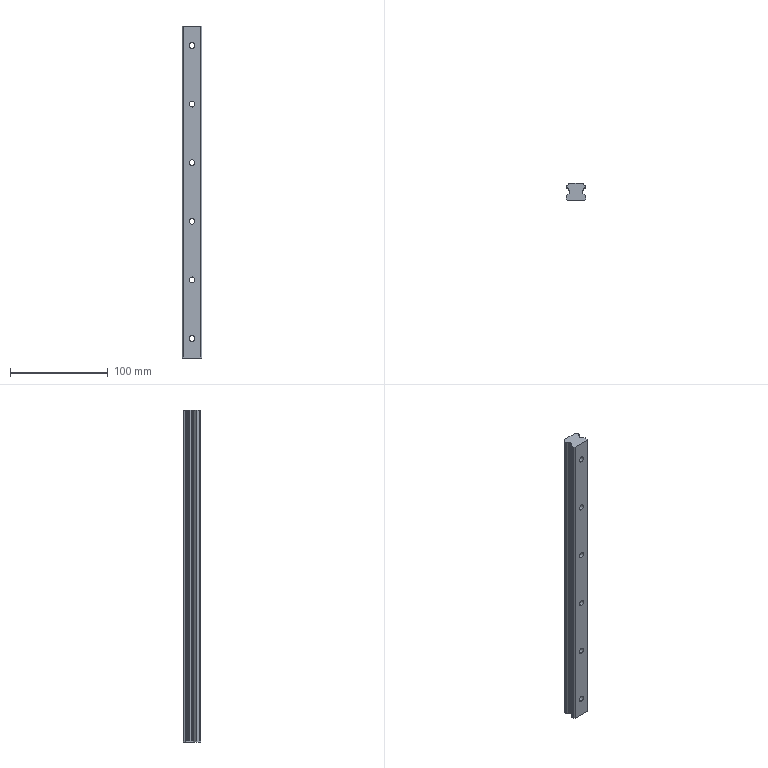Part | SolidWorks | features BaseBody 1 | 1 solid | 74 faces | box 20 x 17.5 x 340 mm | volume 96486 mm3 | cylinder 46 | plane 28 | commonest cylinder face diameters 1 x12 6 x12 9.5 x12 2 x6 4.06 x4